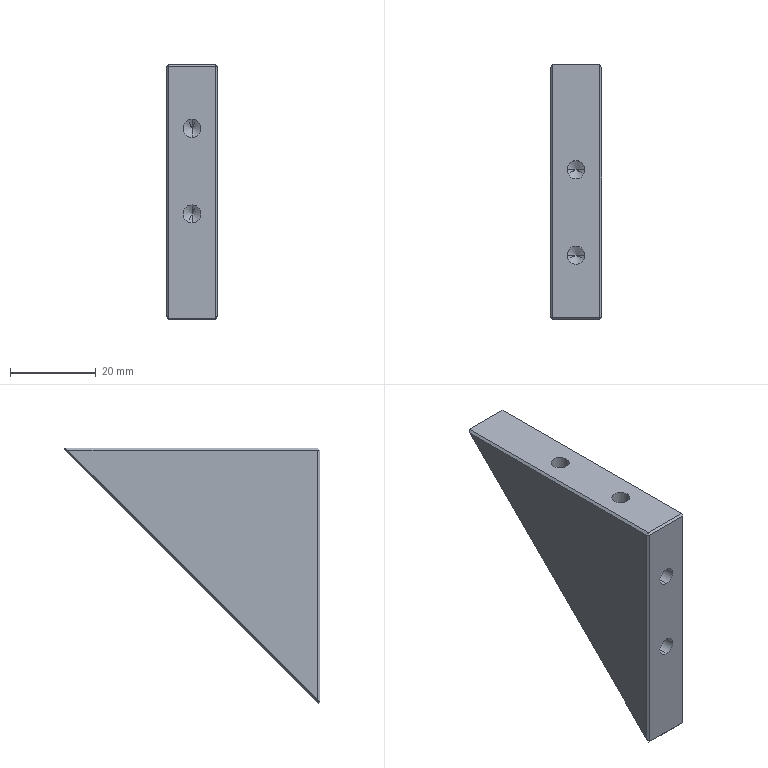Part | STEP file | 06-31 Dovetail fixing triangle plate | 1 solid | 36 faces | box 12 x 59.646 x 59.75 mm | volume 20836 mm3 | plane 20 | cylinder 8 | cone 8 | commonest cylinder face diameters 4.2 x8